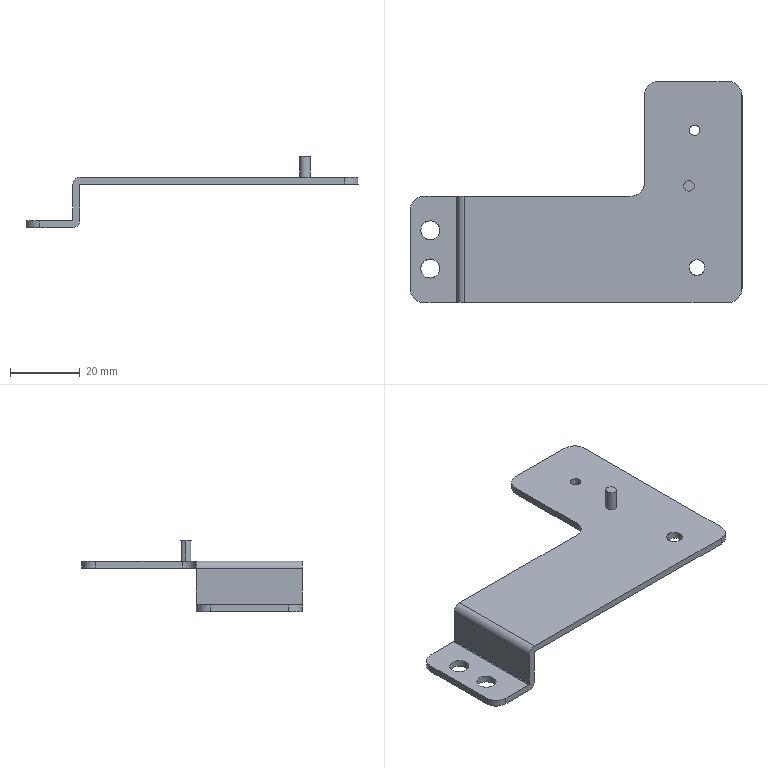Part | NX | features BREP 1 | 1 solid | 31 faces | box 95.45 x 63.5 x 20.5 mm | volume 8247 mm3 | cylinder 18 | plane 13 | commonest cylinder face diameters 8 x6 3 x4 0.3 x2 4.3 x2 4.5 x2 5.5 x2
STEP:
#1=CARTESIAN_POINT('',(-456.8,35.5,220.4));
#2=VERTEX_POINT('',#1);
#3=CARTESIAN_POINT('',(-456.8,35.5,226.4));
#4=VERTEX_POINT('',#3);
#5=CARTESIAN_POINT('',(-456.8,35.5,223.4));
#6=DIRECTION('',(0.,0.,1.));
#7=VECTOR('',#6,1000.);
#8=LINE('',#5,#7);
#9=EDGE_CURVE('',#2,#4,#8,.T.);
#10=ORIENTED_EDGE('',*,*,#9,.F.);
#11=CARTESIAN_POINT('',(-459.8,35.5,220.4));
#12=VERTEX_POINT('',#11);
#13=CARTESIAN_POINT('',(-458.3,35.5,220.4));
#14=DIRECTION('',(0.,0.,1.));
#15=DIRECTION('',(1.,0.,0.));
#16=AXIS2_PLACEMENT_3D('',#13,#14,#15);
#17=CIRCLE('',#16,1.5);
#18=EDGE_CURVE('',#2,#12,#17,.T.);
#19=ORIENTED_EDGE('',*,*,#18,.T.);
#20=CARTESIAN_POINT('',(-459.8,35.5,226.4));
#21=VERTEX_POINT('',#20);
#22=CARTESIAN_POINT('',(-459.8,35.5,223.4));
#23=DIRECTION('',(0.,0.,1.));
#24=VECTOR('',#23,1000.);
#25=LINE('',#22,#24);
#26=EDGE_CURVE('',#12,#21,#25,.T.);
#27=ORIENTED_EDGE('',*,*,#26,.T.);
#28=CARTESIAN_POINT('',(-458.3,35.5,226.4));
#29=DIRECTION('',(0.,0.,1.));
#30=DIRECTION('',(1.,0.,0.));
#31=AXIS2_PLACEMENT_3D('',#28,#29,#30);
#32=CIRCLE('',#31,1.5);
#33=EDGE_CURVE('',#4,#21,#32,.T.);
#34=ORIENTED_EDGE('',*,*,#33,.F.);
#35=EDGE_LOOP('',(#10,#19,#27,#34));
#36=FACE_BOUND('',#35,.T.);
#37=CARTESIAN_POINT('',(-458.3,35.5,223.4));
#38=DIRECTION('',(0.,0.,1.));
#39=DIRECTION('',(1.,0.,0.));
#40=AXIS2_PLACEMENT_3D('',#37,#38,#39);
#41=CYLINDRICAL_SURFACE('',#40,1.5);
#42=ADVANCED_FACE('',(#36),#41,.T.);
#43=ORIENTED_EDGE('',*,*,#26,.F.);
#44=CARTESIAN_POINT('',(-458.3,35.5,220.4));
#45=DIRECTION('',(0.,0.,1.));
#46=DIRECTION('',(1.,0.,0.));
#47=AXIS2_PLACEMENT_3D('',#44,#45,#46);
#48=CIRCLE('',#47,1.5);
#49=EDGE_CURVE('',#12,#2,#48,.T.);
#50=ORIENTED_EDGE('',*,*,#49,.T.);
#51=ORIENTED_EDGE('',*,*,#9,.T.);
#52=CARTESIAN_POINT('',(-458.3,35.5,226.4));
#53=DIRECTION('',(0.,0.,1.));
#54=DIRECTION('',(1.,0.,0.));
#55=AXIS2_PLACEMENT_3D('',#52,#53,#54);
#56=CIRCLE('',#55,1.5);
#57=EDGE_CURVE('',#21,#4,#56,.T.);
#58=ORIENTED_EDGE('',*,*,#57,.F.);
#59=EDGE_LOOP('',(#43,#50,#51,#58));
#60=FACE_BOUND('',#59,.T.);
#61=CARTESIAN_POINT('',(-458.3,35.5,223.4));
#62=DIRECTION('',(0.,0.,1.));
#63=DIRECTION('',(1.,0.,0.));
#64=AXIS2_PLACEMENT_3D('',#61,#62,#63);
#65=CYLINDRICAL_SURFACE('',#64,1.5);
#66=ADVANCED_FACE('',(#60),#65,.T.);
#67=ORIENTED_EDGE('',*,*,#33,.T.);
#68=ORIENTED_EDGE('',*,*,#57,.T.);
#69=EDGE_LOOP('',(#67,#68));
#70=FACE_BOUND('',#69,.T.);
#71=CARTESIAN_POINT('',(0.,0.,226.4));
#72=DIRECTION('',(0.,0.,1.));
#73=DIRECTION('',(1.,0.,0.));
#74=AXIS2_PLACEMENT_3D('',#71,#72,#73);
#75=PLANE('',#74);
#76=ADVANCED_FACE('',(#70),#75,.T.);
#77=CARTESIAN_POINT('',(-443.05,61.5,220.4));
#78=VERTEX_POINT('',#77);
#79=CARTESIAN_POINT('',(-447.05,65.5,220.4));
#80=VERTEX_POINT('',#79);
#81=CARTESIAN_POINT('',(-447.05,61.5,220.4));
#82=DIRECTION('',(0.,0.,1.));
#83=DIRECTION('',(1.,0.,0.));
#84=AXIS2_PLACEMENT_3D('',#81,#82,#83);
#85=CIRCLE('',#84,4.);
#86=EDGE_CURVE('',#78,#80,#85,.T.);
#87=ORIENTED_EDGE('',*,*,#86,.T.);
#88=CARTESIAN_POINT('',(-467.05,65.5,220.4));
#89=VERTEX_POINT('',#88);
#90=CARTESIAN_POINT('',(-457.05,65.5,220.4));
#91=DIRECTION('',(1.,0.,0.));
#92=VECTOR('',#91,1000.);
#93=LINE('',#90,#92);
#94=EDGE_CURVE('',#89,#80,#93,.T.);
#95=ORIENTED_EDGE('',*,*,#94,.F.);
#96=CARTESIAN_POINT('',(-471.05,61.5,220.4));
#97=VERTEX_POINT('',#96);
#98=CARTESIAN_POINT('',(-467.05,61.5,220.4));
#99=DIRECTION('',(0.,0.,1.));
#100=DIRECTION('',(1.,0.,0.));
#101=AXIS2_PLACEMENT_3D('',#98,#99,#100);
#102=CIRCLE('',#101,4.);
#103=EDGE_CURVE('',#89,#97,#102,.T.);
#104=ORIENTED_EDGE('',*,*,#103,.T.);
#105=CARTESIAN_POINT('',(-471.05,36.5,220.4));
#106=VERTEX_POINT('',#105);
#107=CARTESIAN_POINT('',(-471.05,49.,220.4));
#108=DIRECTION('',(0.,-1.,0.));
#109=VECTOR('',#108,1000.);
#110=LINE('',#107,#109);
#111=EDGE_CURVE('',#97,#106,#110,.T.);
#112=ORIENTED_EDGE('',*,*,#111,.T.);
#113=CARTESIAN_POINT('',(-475.05,32.5,220.4));
#114=VERTEX_POINT('',#113);
#115=CARTESIAN_POINT('',(-471.05,36.5,220.4));
#116=CARTESIAN_POINT('',(-471.05,36.108,220.4));
#117=CARTESIAN_POINT('',(-471.098,35.716,220.4));
#118=CARTESIAN_POINT('',(-471.194,35.332,220.4));
#119=CARTESIAN_POINT('',(-471.478,34.595,220.4));
#120=CARTESIAN_POINT('',(-471.932,33.949,220.4));
#121=CARTESIAN_POINT('',(-472.197,33.655,220.4));
#122=CARTESIAN_POINT('',(-472.794,33.139,220.4));
#123=CARTESIAN_POINT('',(-473.499,32.782,220.4));
#124=CARTESIAN_POINT('',(-473.871,32.647,220.4));
#125=CARTESIAN_POINT('',(-474.336,32.542,220.4));
#126=CARTESIAN_POINT('',(-474.807,32.506,220.4));
#127=CARTESIAN_POINT('',(-474.888,32.502,220.4));
#128=CARTESIAN_POINT('',(-474.969,32.5,220.4));
#129=CARTESIAN_POINT('',(-475.05,32.5,220.4));
#130=B_SPLINE_CURVE_WITH_KNOTS('',5,(#115,#116,#117,#118,#119,#120,#121,#122,#123,#124,#125,#126,#127,#128,#129),.UNSPECIFIED.,.F.,.F.,(6,3,3,3,6),(0.,0.3119,0.6238,0.9356,1.),.UNSPECIFIED.);
#131=EDGE_CURVE('',#106,#114,#130,.T.);
#132=ORIENTED_EDGE('',*,*,#131,.T.);
#133=CARTESIAN_POINT('',(-522.85,32.5,220.4));
#134=VERTEX_POINT('',#133);
#135=CARTESIAN_POINT('',(-494.95,32.5,220.4));
#136=DIRECTION('',(1.,0.,0.));
#137=VECTOR('',#136,1000.);
#138=LINE('',#135,#137);
#139=EDGE_CURVE('',#134,#114,#138,.T.);
#140=ORIENTED_EDGE('',*,*,#139,.F.);
#141=CARTESIAN_POINT('',(-522.85,2.,220.4));
#142=VERTEX_POINT('',#141);
#143=CARTESIAN_POINT('',(-522.85,17.25,220.4));
#144=DIRECTION('',(0.,1.,0.));
#145=VECTOR('',#144,1000.);
#146=LINE('',#143,#145);
#147=EDGE_CURVE('',#142,#134,#146,.T.);
#148=ORIENTED_EDGE('',*,*,#147,.F.);
#149=CARTESIAN_POINT('',(-447.05,2.,220.4));
#150=VERTEX_POINT('',#149);
#151=CARTESIAN_POINT('',(-480.95,2.,220.4));
#152=DIRECTION('',(-1.,0.,0.));
#153=VECTOR('',#152,1000.);
#154=LINE('',#151,#153);
#155=EDGE_CURVE('',#150,#142,#154,.T.);
#156=ORIENTED_EDGE('',*,*,#155,.F.);
#157=CARTESIAN_POINT('',(-443.05,6.,220.4));
#158=VERTEX_POINT('',#157);
#159=CARTESIAN_POINT('',(-447.05,6.,220.4));
#160=DIRECTION('',(0.,0.,1.));
#161=DIRECTION('',(1.,0.,0.));
#162=AXIS2_PLACEMENT_3D('',#159,#160,#161);
#163=CIRCLE('',#162,4.);
#164=EDGE_CURVE('',#150,#158,#163,.T.);
#165=ORIENTED_EDGE('',*,*,#164,.T.);
#166=CARTESIAN_POINT('',(-443.05,33.75,220.4));
#167=DIRECTION('',(0.,1.,0.));
#168=VECTOR('',#167,1000.);
#169=LINE('',#166,#168);
#170=EDGE_CURVE('',#158,#78,#169,.T.);
#171=ORIENTED_EDGE('',*,*,#170,.T.);
#172=EDGE_LOOP('',(#87,#95,#104,#112,#132,#140,#148,#156,#165,#171));
#173=FACE_BOUND('',#172,.T.);
#174=ORIENTED_EDGE('',*,*,#18,.F.);
#175=ORIENTED_EDGE('',*,*,#49,.F.);
#176=EDGE_LOOP('',(#174,#175));
#177=FACE_BOUND('',#176,.T.);
#178=CARTESIAN_POINT('',(-458.25,12.,220.4));
#179=VERTEX_POINT('',#178);
#180=CARTESIAN_POINT('',(-453.75,12.,220.4));
#181=VERTEX_POINT('',#180);
#182=CARTESIAN_POINT('',(-458.25,12.,220.4));
#183=CARTESIAN_POINT('',(-458.25,12.22,220.4));
#184=CARTESIAN_POINT('',(-458.223,12.441,220.4));
#185=CARTESIAN_POINT('',(-458.169,12.657,220.4));
#186=CARTESIAN_POINT('',(-458.009,13.071,220.4));
#187=CARTESIAN_POINT('',(-457.754,13.435,220.4));
#188=CARTESIAN_POINT('',(-457.605,13.6,220.4));
#189=CARTESIAN_POINT('',(-457.269,13.891,220.4));
#190=CARTESIAN_POINT('',(-456.873,14.092,220.4));
#191=CARTESIAN_POINT('',(-456.663,14.167,220.4));
#192=CARTESIAN_POINT('',(-456.23,14.265,220.4));
#193=CARTESIAN_POINT('',(-455.786,14.256,220.4));
#194=CARTESIAN_POINT('',(-455.565,14.224,220.4));
#195=CARTESIAN_POINT('',(-455.137,14.107,220.4));
#196=CARTESIAN_POINT('',(-454.749,13.89,220.4));
#197=CARTESIAN_POINT('',(-454.57,13.758,220.4));
#198=CARTESIAN_POINT('',(-454.247,13.453,220.4));
#199=CARTESIAN_POINT('',(-454.007,13.079,220.4));
#200=CARTESIAN_POINT('',(-453.911,12.878,220.4));
#201=CARTESIAN_POINT('',(-453.811,12.581,220.4));
#202=CARTESIAN_POINT('',(-453.764,12.273,220.4));
#203=CARTESIAN_POINT('',(-453.755,12.182,220.4));
#204=CARTESIAN_POINT('',(-453.75,12.091,220.4));
#205=CARTESIAN_POINT('',(-453.75,12.,220.4));
#206=B_SPLINE_CURVE_WITH_KNOTS('',5,(#182,#183,#184,#185,#186,#187,#188,#189,#190,#191,#192,#193,#194,#195,#196,#197,#198,#199,#200,#201,#202,#203,#204,#205),.UNSPECIFIED.,.F.,.F.,(6,3,3,3,3,3,3,6),(0.,0.156,0.3119,0.4679,0.6238,0.7798,0.9357,1.),.UNSPECIFIED.);
#207=EDGE_CURVE('',#179,#181,#206,.T.);
#208=ORIENTED_EDGE('',*,*,#207,.T.);
#209=CARTESIAN_POINT('',(-453.75,12.,220.4));
#210=CARTESIAN_POINT('',(-453.75,11.78,220.4));
#211=CARTESIAN_POINT('',(-453.777,11.559,220.4));
#212=CARTESIAN_POINT('',(-453.831,11.343,220.4));
#213=CARTESIAN_POINT('',(-453.991,10.929,220.4));
#214=CARTESIAN_POINT('',(-454.246,10.565,220.4));
#215=CARTESIAN_POINT('',(-454.395,10.4,220.4));
#216=CARTESIAN_POINT('',(-454.731,10.109,220.4));
#217=CARTESIAN_POINT('',(-455.127,9.908,220.4));
#218=CARTESIAN_POINT('',(-455.337,9.833,220.4));
#219=CARTESIAN_POINT('',(-455.77,9.735,220.4));
#220=CARTESIAN_POINT('',(-456.214,9.744,220.4));
#221=CARTESIAN_POINT('',(-456.435,9.776,220.4));
#222=CARTESIAN_POINT('',(-456.863,9.893,220.4));
#223=CARTESIAN_POINT('',(-457.251,10.11,220.4));
#224=CARTESIAN_POINT('',(-457.43,10.242,220.4));
#225=CARTESIAN_POINT('',(-457.753,10.547,220.4));
#226=CARTESIAN_POINT('',(-457.993,10.921,220.4));
#227=CARTESIAN_POINT('',(-458.089,11.122,220.4));
#228=CARTESIAN_POINT('',(-458.189,11.419,220.4));
#229=CARTESIAN_POINT('',(-458.236,11.727,220.4));
#230=CARTESIAN_POINT('',(-458.245,11.818,220.4));
#231=CARTESIAN_POINT('',(-458.25,11.909,220.4));
#232=CARTESIAN_POINT('',(-458.25,12.,220.4));
#233=B_SPLINE_CURVE_WITH_KNOTS('',5,(#209,#210,#211,#212,#213,#214,#215,#216,#217,#218,#219,#220,#221,#222,#223,#224,#225,#226,#227,#228,#229,#230,#231,#232),.UNSPECIFIED.,.F.,.F.,(6,3,3,3,3,3,3,6),(0.,0.156,0.3119,0.4679,0.6238,0.7798,0.9357,1.),.UNSPECIFIED.);
#234=EDGE_CURVE('',#181,#179,#233,.T.);
#235=ORIENTED_EDGE('',*,*,#234,.T.);
#236=EDGE_LOOP('',(#208,#235));
#237=FACE_BOUND('',#236,.T.);
#238=CARTESIAN_POINT('',(-457.991,52.219,220.4));
#239=VERTEX_POINT('',#238);
#240=CARTESIAN_POINT('',(-455.359,50.781,220.4));
#241=VERTEX_POINT('',#240);
#242=CARTESIAN_POINT('',(-457.991,52.219,220.4));
#243=CARTESIAN_POINT('',(-457.905,52.377,220.4));
#244=CARTESIAN_POINT('',(-457.795,52.522,220.4));
#245=CARTESIAN_POINT('',(-457.664,52.649,220.4));
#246=CARTESIAN_POINT('',(-457.368,52.861,220.4));
#247=CARTESIAN_POINT('',(-457.022,52.976,220.4));
#248=CARTESIAN_POINT('',(-456.842,53.007,220.4));
#249=CARTESIAN_POINT('',(-456.478,53.014,220.4));
#250=CARTESIAN_POINT('',(-456.128,52.914,220.4));
#251=CARTESIAN_POINT('',(-455.962,52.838,220.4));
#252=CARTESIAN_POINT('',(-455.658,52.639,220.4));
#253=CARTESIAN_POINT('',(-455.425,52.359,220.4));
#254=CARTESIAN_POINT('',(-455.331,52.202,220.4));
#255=CARTESIAN_POINT('',(-455.192,51.865,220.4));
#256=CARTESIAN_POINT('',(-455.159,51.503,220.4));
#257=CARTESIAN_POINT('',(-455.169,51.32,220.4));
#258=CARTESIAN_POINT('',(-455.216,51.1,220.4));
#259=CARTESIAN_POINT('',(-455.302,50.895,220.4));
#260=CARTESIAN_POINT('',(-455.319,50.856,220.4));
#261=CARTESIAN_POINT('',(-455.338,50.818,220.4));
#262=CARTESIAN_POINT('',(-455.359,50.781,220.4));
#263=B_SPLINE_CURVE_WITH_KNOTS('',5,(#242,#243,#244,#245,#246,#247,#248,#249,#250,#251,#252,#253,#254,#255,#256,#257,#258,#259,#260,#261,#262),.UNSPECIFIED.,.F.,.F.,(6,3,3,3,3,3,6),(0.,0.191,0.382,0.573,0.764,0.9549,1.),.UNSPECIFIED.);
#264=EDGE_CURVE('',#239,#241,#263,.T.);
#265=ORIENTED_EDGE('',*,*,#264,.T.);
#266=CARTESIAN_POINT('',(-455.359,50.781,220.4));
#267=CARTESIAN_POINT('',(-455.445,50.623,220.4));
#268=CARTESIAN_POINT('',(-455.555,50.478,220.4));
#269=CARTESIAN_POINT('',(-455.686,50.351,220.4));
#270=CARTESIAN_POINT('',(-455.982,50.139,220.4));
#271=CARTESIAN_POINT('',(-456.328,50.024,220.4));
#272=CARTESIAN_POINT('',(-456.508,49.993,220.4));
#273=CARTESIAN_POINT('',(-456.872,49.986,220.4));
#274=CARTESIAN_POINT('',(-457.222,50.086,220.4));
#275=CARTESIAN_POINT('',(-457.388,50.162,220.4));
#276=CARTESIAN_POINT('',(-457.692,50.361,220.4));
#277=CARTESIAN_POINT('',(-457.925,50.641,220.4));
#278=CARTESIAN_POINT('',(-458.019,50.798,220.4));
#279=CARTESIAN_POINT('',(-458.158,51.135,220.4));
#280=CARTESIAN_POINT('',(-458.191,51.497,220.4));
#281=CARTESIAN_POINT('',(-458.181,51.68,220.4));
#282=CARTESIAN_POINT('',(-458.134,51.9,220.4));
#283=CARTESIAN_POINT('',(-458.048,52.105,220.4));
#284=CARTESIAN_POINT('',(-458.031,52.144,220.4));
#285=CARTESIAN_POINT('',(-458.012,52.182,220.4));
#286=CARTESIAN_POINT('',(-457.991,52.219,220.4));
#287=B_SPLINE_CURVE_WITH_KNOTS('',5,(#266,#267,#268,#269,#270,#271,#272,#273,#274,#275,#276,#277,#278,#279,#280,#281,#282,#283,#284,#285,#286),.UNSPECIFIED.,.F.,.F.,(6,3,3,3,3,3,6),(0.,0.191,0.382,0.573,0.764,0.9549,1.),.UNSPECIFIED.);
#288=EDGE_CURVE('',#241,#239,#287,.T.);
#289=ORIENTED_EDGE('',*,*,#288,.T.);
#290=EDGE_LOOP('',(#265,#289));
#291=FACE_BOUND('',#290,.T.);
#292=CARTESIAN_POINT('',(0.,0.,220.4));
#293=DIRECTION('',(0.,0.,1.));
#294=DIRECTION('',(-1.,0.,0.));
#295=AXIS2_PLACEMENT_3D('',#292,#293,#294);
#296=PLANE('',#295);
#297=ADVANCED_FACE('',(#173,#177,#237,#291),#296,.T.);
#298=CARTESIAN_POINT('',(-535.433,11.75,205.9));
#299=VERTEX_POINT('',#298);
#300=CARTESIAN_POINT('',(-532.683,11.75,205.9));
#301=DIRECTION('',(0.,0.,-1.));
#302=DIRECTION('',(-1.,0.,0.));
#303=AXIS2_PLACEMENT_3D('',#300,#301,#302);
#304=CIRCLE('',#303,2.75);
#305=EDGE_CURVE('',#299,#299,#304,.T.);
#306=ORIENTED_EDGE('',*,*,#305,.F.);
#307=EDGE_LOOP('',(#306));
#308=FACE_BOUND('',#307,.T.);
#309=CARTESIAN_POINT('',(-535.433,22.75,205.9));
#310=VERTEX_POINT('',#309);
#311=CARTESIAN_POINT('',(-532.683,22.75,205.9));
#312=DIRECTION('',(0.,0.,-1.));
#313=DIRECTION('',(-1.,0.,0.));
#314=AXIS2_PLACEMENT_3D('',#311,#312,#313);
#315=CIRCLE('',#314,2.75);
#316=EDGE_CURVE('',#310,#310,#315,.T.);
#317=ORIENTED_EDGE('',*,*,#316,.F.);
#318=EDGE_LOOP('',(#317));
#319=FACE_BOUND('',#318,.T.);
#320=CARTESIAN_POINT('',(-538.5,28.5,205.9));
#321=VERTEX_POINT('',#320);
#322=CARTESIAN_POINT('',(-534.5,32.5,205.9));
#323=VERTEX_POINT('',#322);
#324=CARTESIAN_POINT('',(-534.5,28.5,205.9));
#325=DIRECTION('',(0.,0.,-1.));
#326=DIRECTION('',(-1.,0.,0.));
#327=AXIS2_PLACEMENT_3D('',#324,#325,#326);
#328=CIRCLE('',#327,4.);
#329=EDGE_CURVE('',#321,#323,#328,.T.);
#330=ORIENTED_EDGE('',*,*,#329,.T.);
#331=CARTESIAN_POINT('',(-525.15,32.5,205.9));
#332=VERTEX_POINT('',#331);
#333=CARTESIAN_POINT('',(-531.075,32.5,205.9));
#334=DIRECTION('',(-1.,0.,0.));
#335=VECTOR('',#334,1000.);
#336=LINE('',#333,#335);
#337=EDGE_CURVE('',#332,#323,#336,.T.);
#338=ORIENTED_EDGE('',*,*,#337,.F.);
#339=CARTESIAN_POINT('',(-525.15,2.,205.9));
#340=VERTEX_POINT('',#339);
#341=CARTESIAN_POINT('',(-525.15,0.,205.9));
#342=DIRECTION('',(0.,1.,0.));
#343=VECTOR('',#342,1000.);
#344=LINE('',#341,#343);
#345=EDGE_CURVE('',#340,#332,#344,.T.);
#346=ORIENTED_EDGE('',*,*,#345,.F.);
#347=CARTESIAN_POINT('',(-534.5,2.,205.9));
#348=VERTEX_POINT('',#347);
#349=CARTESIAN_POINT('',(-531.075,2.,205.9));
#350=DIRECTION('',(1.,0.,0.));
#351=VECTOR('',#350,1000.);
#352=LINE('',#349,#351);
#353=EDGE_CURVE('',#348,#340,#352,.T.);
#354=ORIENTED_EDGE('',*,*,#353,.F.);
#355=CARTESIAN_POINT('',(-538.5,6.,205.9));
#356=VERTEX_POINT('',#355);
#357=CARTESIAN_POINT('',(-534.5,6.,205.9));
#358=DIRECTION('',(0.,0.,-1.));
#359=DIRECTION('',(-1.,0.,0.));
#360=AXIS2_PLACEMENT_3D('',#357,#358,#359);
#361=CIRCLE('',#360,4.);
#362=EDGE_CURVE('',#348,#356,#361,.T.);
#363=ORIENTED_EDGE('',*,*,#362,.T.);
#364=CARTESIAN_POINT('',(-538.5,17.25,205.9));
#365=DIRECTION('',(0.,-1.,0.));
#366=VECTOR('',#365,1000.);
#367=LINE('',#364,#366);
#368=EDGE_CURVE('',#321,#356,#367,.T.);
#369=ORIENTED_EDGE('',*,*,#368,.F.);
#370=EDGE_LOOP('',(#330,#338,#346,#354,#363,#369));
#371=FACE_BOUND('',#370,.T.);
#372=CARTESIAN_POINT('',(-8.,0.,205.9));
#373=DIRECTION('',(0.,0.,-1.));
#374=DIRECTION('',(0.,1.,0.));
#375=AXIS2_PLACEMENT_3D('',#372,#373,#374);
#376=PLANE('',#375);
#377=ADVANCED_FACE('',(#308,#319,#371),#376,.T.);
#378=CARTESIAN_POINT('',(-538.5,28.5,207.9));
#379=VERTEX_POINT('',#378);
#380=CARTESIAN_POINT('',(-538.5,28.5,205.9));
#381=DIRECTION('',(0.,0.,1.));
#382=VECTOR('',#381,1000.);
#383=LINE('',#380,#382);
#384=EDGE_CURVE('',#321,#379,#383,.T.);
#385=ORIENTED_EDGE('',*,*,#384,.F.);
#386=ORIENTED_EDGE('',*,*,#368,.T.);
#387=CARTESIAN_POINT('',(-538.5,6.,207.9));
#388=VERTEX_POINT('',#387);
#389=CARTESIAN_POINT('',(-538.5,6.,206.9));
#390=DIRECTION('',(0.,0.,-1.));
#391=VECTOR('',#390,1000.);
#392=LINE('',#389,#391);
#393=EDGE_CURVE('',#388,#356,#392,.T.);
#394=ORIENTED_EDGE('',*,*,#393,.F.);
#395=CARTESIAN_POINT('',(-538.5,17.25,207.9));
#396=DIRECTION('',(0.,-1.,0.));
#397=VECTOR('',#396,1000.);
#398=LINE('',#395,#397);
#399=EDGE_CURVE('',#379,#388,#398,.T.);
#400=ORIENTED_EDGE('',*,*,#399,.F.);
#401=EDGE_LOOP('',(#385,#386,#394,#400));
#402=FACE_BOUND('',#401,.T.);
#403=CARTESIAN_POINT('',(-538.5,2.,205.9));
#404=DIRECTION('',(1.,0.,0.));
#405=DIRECTION('',(0.,-1.,0.));
#406=AXIS2_PLACEMENT_3D('',#403,#404,#405);
#407=PLANE('',#406);
#408=ADVANCED_FACE('',(#402),#407,.F.);
#409=ORIENTED_EDGE('',*,*,#384,.T.);
#410=CARTESIAN_POINT('',(-534.5,32.5,207.9));
#411=VERTEX_POINT('',#410);
#412=CARTESIAN_POINT('',(-534.5,28.5,207.9));
#413=DIRECTION('',(0.,0.,1.));
#414=DIRECTION('',(-1.,0.,0.));
#415=AXIS2_PLACEMENT_3D('',#412,#413,#414);
#416=CIRCLE('',#415,4.);
#417=EDGE_CURVE('',#411,#379,#416,.T.);
#418=ORIENTED_EDGE('',*,*,#417,.F.);
#419=CARTESIAN_POINT('',(-534.5,32.5,228.4));
#420=DIRECTION('',(0.,0.,-1.));
#421=VECTOR('',#420,1000.);
#422=LINE('',#419,#421);
#423=EDGE_CURVE('',#411,#323,#422,.T.);
#424=ORIENTED_EDGE('',*,*,#423,.T.);
#425=ORIENTED_EDGE('',*,*,#329,.F.);
#426=EDGE_LOOP('',(#409,#418,#424,#425));
#427=FACE_BOUND('',#426,.T.);
#428=CARTESIAN_POINT('',(-534.5,28.5,205.9));
#429=DIRECTION('',(0.,0.,1.));
#430=DIRECTION('',(-1.,0.,0.));
#431=AXIS2_PLACEMENT_3D('',#428,#429,#430);
#432=CYLINDRICAL_SURFACE('',#431,4.);
#433=ADVANCED_FACE('',(#427),#432,.T.);
#434=CARTESIAN_POINT('',(-523.,32.5,208.05));
#435=VERTEX_POINT('',#434);
#436=CARTESIAN_POINT('',(-523.,2.,208.05));
#437=VERTEX_POINT('',#436);
#438=CARTESIAN_POINT('',(-523.,0.,208.05));
#439=DIRECTION('',(0.,-1.,0.));
#440=VECTOR('',#439,1000.);
#441=LINE('',#438,#440);
#442=EDGE_CURVE('',#435,#437,#441,.T.);
#443=ORIENTED_EDGE('',*,*,#442,.F.);
#444=CARTESIAN_POINT('',(-523.,32.5,218.25));
#445=VERTEX_POINT('',#444);
#446=CARTESIAN_POINT('',(-523.,32.5,208.15));
#447=DIRECTION('',(0.,0.,-1.));
#448=VECTOR('',#447,1000.);
#449=LINE('',#446,#448);
#450=EDGE_CURVE('',#445,#435,#449,.T.);
#451=ORIENTED_EDGE('',*,*,#450,.F.);
#452=CARTESIAN_POINT('',(-523.,2.,218.25));
#453=VERTEX_POINT('',#452);
#454=CARTESIAN_POINT('',(-523.,0.,218.25));
#455=DIRECTION('',(0.,1.,0.));
#456=VECTOR('',#455,1000.);
#457=LINE('',#454,#456);
#458=EDGE_CURVE('',#453,#445,#457,.T.);
#459=ORIENTED_EDGE('',*,*,#458,.F.);
#460=CARTESIAN_POINT('',(-523.,2.,208.15));
#461=DIRECTION('',(0.,0.,1.));
#462=VECTOR('',#461,1000.);
#463=LINE('',#460,#462);
#464=EDGE_CURVE('',#437,#453,#463,.T.);
#465=ORIENTED_EDGE('',*,*,#464,.F.);
#466=EDGE_LOOP('',(#443,#451,#459,#465));
#467=FACE_BOUND('',#466,.T.);
#468=CARTESIAN_POINT('',(-523.,0.,0.));
#469=DIRECTION('',(1.,0.,0.));
#470=DIRECTION('',(0.,-1.,0.));
#471=AXIS2_PLACEMENT_3D('',#468,#469,#470);
#472=PLANE('',#471);
#473=ADVANCED_FACE('',(#467),#472,.T.);
#474=CARTESIAN_POINT('',(-525.15,2.,208.05));
#475=DIRECTION('',(0.,-1.,0.));
#476=DIRECTION('',(0.,0.,-1.));
#477=AXIS2_PLACEMENT_3D('',#474,#475,#476);
#478=CIRCLE('',#477,2.15);
#479=EDGE_CURVE('',#340,#437,#478,.T.);
#480=ORIENTED_EDGE('',*,*,#479,.F.);
#481=ORIENTED_EDGE('',*,*,#345,.T.);
#482=CARTESIAN_POINT('',(-525.15,32.5,208.05));
#483=DIRECTION('',(0.,1.,0.));
#484=DIRECTION('',(0.,0.,1.));
#485=AXIS2_PLACEMENT_3D('',#482,#483,#484);
#486=CIRCLE('',#485,2.15);
#487=EDGE_CURVE('',#435,#332,#486,.T.);
#488=ORIENTED_EDGE('',*,*,#487,.F.);
#489=ORIENTED_EDGE('',*,*,#442,.T.);
#490=EDGE_LOOP('',(#480,#481,#488,#489));
#491=FACE_BOUND('',#490,.T.);
#492=CARTESIAN_POINT('',(-525.15,0.,208.05));
#493=DIRECTION('',(0.,-1.,0.));
#494=DIRECTION('',(0.,0.,-1.));
#495=AXIS2_PLACEMENT_3D('',#492,#493,#494);
#496=CYLINDRICAL_SURFACE('',#495,2.15);
#497=ADVANCED_FACE('',(#491),#496,.T.);
#498=CARTESIAN_POINT('',(-534.5,2.,207.9));
#499=VERTEX_POINT('',#498);
#500=CARTESIAN_POINT('',(-534.5,2.,205.9));
#501=DIRECTION('',(0.,0.,1.));
#502=VECTOR('',#501,1000.);
#503=LINE('',#500,#502);
#504=EDGE_CURVE('',#348,#499,#503,.T.);
#505=ORIENTED_EDGE('',*,*,#504,.T.);
#506=CARTESIAN_POINT('',(-534.5,6.,207.9));
#507=DIRECTION('',(0.,0.,1.));
#508=DIRECTION('',(-1.,0.,0.));
#509=AXIS2_PLACEMENT_3D('',#506,#507,#508);
#510=CIRCLE('',#509,4.);
#511=EDGE_CURVE('',#388,#499,#510,.T.);
#512=ORIENTED_EDGE('',*,*,#511,.F.);
#513=ORIENTED_EDGE('',*,*,#393,.T.);
#514=ORIENTED_EDGE('',*,*,#362,.F.);
#515=EDGE_LOOP('',(#505,#512,#513,#514));
#516=FACE_BOUND('',#515,.T.);
#517=CARTESIAN_POINT('',(-534.5,6.,205.9));
#518=DIRECTION('',(0.,0.,-1.));
#519=DIRECTION('',(1.,0.,0.));
#520=AXIS2_PLACEMENT_3D('',#517,#518,#519);
#521=CYLINDRICAL_SURFACE('',#520,4.);
#522=ADVANCED_FACE('',(#516),#521,.T.);
#523=CARTESIAN_POINT('',(-532.683,9.,207.9));
#524=VERTEX_POINT('',#523);
#525=CARTESIAN_POINT('',(-532.683,11.75,207.9));
#526=DIRECTION('',(0.,0.,1.));
#527=DIRECTION('',(0.,-1.,0.));
#528=AXIS2_PLACEMENT_3D('',#525,#526,#527);
#529=CIRCLE('',#528,2.75);
#530=EDGE_CURVE('',#524,#524,#529,.T.);
#531=ORIENTED_EDGE('',*,*,#530,.F.);
#532=EDGE_LOOP('',(#531));
#533=FACE_BOUND('',#532,.T.);
#534=CARTESIAN_POINT('',(-532.683,20.,207.9));
#535=VERTEX_POINT('',#534);
#536=CARTESIAN_POINT('',(-532.683,22.75,207.9));
#537=DIRECTION('',(0.,0.,1.));
#538=DIRECTION('',(0.,-1.,0.));
#539=AXIS2_PLACEMENT_3D('',#536,#537,#538);
#540=CIRCLE('',#539,2.75);
#541=EDGE_CURVE('',#535,#535,#540,.T.);
#542=ORIENTED_EDGE('',*,*,#541,.F.);
#543=EDGE_LOOP('',(#542));
#544=FACE_BOUND('',#543,.T.);
#545=ORIENTED_EDGE('',*,*,#417,.T.);
#546=ORIENTED_EDGE('',*,*,#399,.T.);
#547=ORIENTED_EDGE('',*,*,#511,.T.);
#548=CARTESIAN_POINT('',(-525.15,2.,207.9));
#549=VERTEX_POINT('',#548);
#550=CARTESIAN_POINT('',(-531.075,2.,207.9));
#551=DIRECTION('',(1.,0.,0.));
#552=VECTOR('',#551,1000.);
#553=LINE('',#550,#552);
#554=EDGE_CURVE('',#499,#549,#553,.T.);
#555=ORIENTED_EDGE('',*,*,#554,.T.);
#556=CARTESIAN_POINT('',(-525.15,32.5,207.9));
#557=VERTEX_POINT('',#556);
#558=CARTESIAN_POINT('',(-525.15,17.25,207.9));
#559=DIRECTION('',(0.,-1.,0.));
#560=VECTOR('',#559,1000.);
#561=LINE('',#558,#560);
#562=EDGE_CURVE('',#557,#549,#561,.T.);
#563=ORIENTED_EDGE('',*,*,#562,.F.);
#564=CARTESIAN_POINT('',(-531.075,32.5,207.9));
#565=DIRECTION('',(-1.,0.,0.));
#566=VECTOR('',#565,1000.);
#567=LINE('',#564,#566);
#568=EDGE_CURVE('',#557,#411,#567,.T.);
#569=ORIENTED_EDGE('',*,*,#568,.T.);
#570=EDGE_LOOP('',(#545,#546,#547,#555,#563,#569));
#571=FACE_BOUND('',#570,.T.);
#572=CARTESIAN_POINT('',(-8.,0.,207.9));
#573=DIRECTION('',(0.,0.,-1.));
#574=DIRECTION('',(0.,1.,0.));
#575=AXIS2_PLACEMENT_3D('',#572,#573,#574);
#576=PLANE('',#575);
#577=ADVANCED_FACE('',(#533,#544,#571),#576,.F.);
#578=CARTESIAN_POINT('',(-525.,32.5,208.05));
#579=VERTEX_POINT('',#578);
#580=CARTESIAN_POINT('',(-525.15,32.5,208.05));
#581=DIRECTION('',(0.,-1.,0.));
#582=DIRECTION('',(1.,0.,0.));
#583=AXIS2_PLACEMENT_3D('',#580,#581,#582);
#584=CIRCLE('',#583,0.15);
#585=EDGE_CURVE('',#557,#579,#584,.T.);
#586=ORIENTED_EDGE('',*,*,#585,.F.);
#587=ORIENTED_EDGE('',*,*,#562,.T.);
#588=CARTESIAN_POINT('',(-525.,2.,208.05));
#589=VERTEX_POINT('',#588);
#590=CARTESIAN_POINT('',(-525.15,2.,208.05));
#591=DIRECTION('',(0.,1.,0.));
#592=DIRECTION('',(1.,0.,0.));
#593=AXIS2_PLACEMENT_3D('',#590,#591,#592);
#594=CIRCLE('',#593,0.15);
#595=EDGE_CURVE('',#589,#549,#594,.T.);
#596=ORIENTED_EDGE('',*,*,#595,.F.);
#597=CARTESIAN_POINT('',(-525.,2.,208.05));
#598=DIRECTION('',(0.,1.,0.));
#599=VECTOR('',#598,1000.);
#600=LINE('',#597,#599);
#601=EDGE_CURVE('',#589,#579,#600,.T.);
#602=ORIENTED_EDGE('',*,*,#601,.T.);
#603=EDGE_LOOP('',(#586,#587,#596,#602));
#604=FACE_BOUND('',#603,.T.);
#605=CARTESIAN_POINT('',(-525.15,2.,208.05));
#606=DIRECTION('',(0.,1.,0.));
#607=DIRECTION('',(1.,0.,0.));
#608=AXIS2_PLACEMENT_3D('',#605,#606,#607);
#609=CYLINDRICAL_SURFACE('',#608,0.15);
#610=ADVANCED_FACE('',(#604),#609,.F.);
#611=CARTESIAN_POINT('',(-525.,2.,218.25));
#612=VERTEX_POINT('',#611);
#613=CARTESIAN_POINT('',(-525.,2.,208.15));
#614=DIRECTION('',(0.,0.,1.));
#615=VECTOR('',#614,1000.);
#616=LINE('',#613,#615);
#617=EDGE_CURVE('',#589,#612,#616,.T.);
#618=ORIENTED_EDGE('',*,*,#617,.T.);
#619=CARTESIAN_POINT('',(-525.,32.5,218.25));
#620=VERTEX_POINT('',#619);
#621=CARTESIAN_POINT('',(-525.,17.25,218.25));
#622=DIRECTION('',(0.,-1.,0.));
#623=VECTOR('',#622,1000.);
#624=LINE('',#621,#623);
#625=EDGE_CURVE('',#620,#612,#624,.T.);
#626=ORIENTED_EDGE('',*,*,#625,.F.);
#627=CARTESIAN_POINT('',(-525.,32.5,208.15));
#628=DIRECTION('',(0.,0.,-1.));
#629=VECTOR('',#628,1000.);
#630=LINE('',#627,#629);
#631=EDGE_CURVE('',#620,#579,#630,.T.);
#632=ORIENTED_EDGE('',*,*,#631,.T.);
#633=ORIENTED_EDGE('',*,*,#601,.F.);
#634=EDGE_LOOP('',(#618,#626,#632,#633));
#635=FACE_BOUND('',#634,.T.);
#636=CARTESIAN_POINT('',(-525.,0.,0.));
#637=DIRECTION('',(1.,0.,0.));
#638=DIRECTION('',(0.,-1.,0.));
#639=AXIS2_PLACEMENT_3D('',#636,#637,#638);
#640=PLANE('',#639);
#641=ADVANCED_FACE('',(#635),#640,.F.);
#642=CARTESIAN_POINT('',(-522.85,32.5,218.25));
#643=DIRECTION('',(0.,1.,0.));
#644=DIRECTION('',(1.,0.,0.));
#645=AXIS2_PLACEMENT_3D('',#642,#643,#644);
#646=CIRCLE('',#645,2.15);
#647=EDGE_CURVE('',#620,#134,#646,.T.);
#648=ORIENTED_EDGE('',*,*,#647,.F.);
#649=ORIENTED_EDGE('',*,*,#625,.T.);
#650=CARTESIAN_POINT('',(-522.85,2.,218.25));
#651=DIRECTION('',(0.,-1.,0.));
#652=DIRECTION('',(1.,0.,0.));
#653=AXIS2_PLACEMENT_3D('',#650,#651,#652);
#654=CIRCLE('',#653,2.15);
#655=EDGE_CURVE('',#142,#612,#654,.T.);
#656=ORIENTED_EDGE('',*,*,#655,.F.);
#657=ORIENTED_EDGE('',*,*,#147,.T.);
#658=EDGE_LOOP('',(#648,#649,#656,#657));
#659=FACE_BOUND('',#658,.T.);
#660=CARTESIAN_POINT('',(-522.85,32.5,218.25));
#661=DIRECTION('',(0.,-1.,0.));
#662=DIRECTION('',(0.,0.,1.));
#663=AXIS2_PLACEMENT_3D('',#660,#661,#662);
#664=CYLINDRICAL_SURFACE('',#663,2.15);
#665=ADVANCED_FACE('',(#659),#664,.T.);
#666=CARTESIAN_POINT('',(-453.75,12.,218.4));
#667=VERTEX_POINT('',#666);
#668=CARTESIAN_POINT('',(-453.75,12.,211.4));
#669=DIRECTION('',(0.,0.,-1.));
#670=VECTOR('',#669,1000.);
#671=LINE('',#668,#670);
#672=EDGE_CURVE('',#181,#667,#671,.T.);
#673=ORIENTED_EDGE('',*,*,#672,.F.);
#674=ORIENTED_EDGE('',*,*,#207,.F.);
#675=CARTESIAN_POINT('',(-458.25,12.,218.4));
#676=VERTEX_POINT('',#675);
#677=CARTESIAN_POINT('',(-458.25,12.,211.4));
#678=DIRECTION('',(0.,0.,1.));
#679=VECTOR('',#678,1000.);
#680=LINE('',#677,#679);
#681=EDGE_CURVE('',#676,#179,#680,.T.);
#682=ORIENTED_EDGE('',*,*,#681,.F.);
#683=CARTESIAN_POINT('',(-456.,12.,218.4));
#684=DIRECTION('',(0.,0.,1.));
#685=DIRECTION('',(1.,0.,0.));
#686=AXIS2_PLACEMENT_3D('',#683,#684,#685);
#687=CIRCLE('',#686,2.25);
#688=EDGE_CURVE('',#667,#676,#687,.T.);
#689=ORIENTED_EDGE('',*,*,#688,.F.);
#690=EDGE_LOOP('',(#673,#674,#682,#689));
#691=FACE_BOUND('',#690,.T.);
#692=CARTESIAN_POINT('',(-456.,12.,211.4));
#693=DIRECTION('',(0.,0.,1.));
#694=DIRECTION('',(1.,0.,0.));
#695=AXIS2_PLACEMENT_3D('',#692,#693,#694);
#696=CYLINDRICAL_SURFACE('',#695,2.25);
#697=ADVANCED_FACE('',(#691),#696,.F.);
#698=ORIENTED_EDGE('',*,*,#681,.T.);
#699=ORIENTED_EDGE('',*,*,#234,.F.);
#700=ORIENTED_EDGE('',*,*,#672,.T.);
#701=CARTESIAN_POINT('',(-456.,12.,218.4));
#702=DIRECTION('',(0.,0.,1.));
#703=DIRECTION('',(1.,0.,0.));
#704=AXIS2_PLACEMENT_3D('',#701,#702,#703);
#705=CIRCLE('',#704,2.25);
#706=EDGE_CURVE('',#676,#667,#705,.T.);
#707=ORIENTED_EDGE('',*,*,#706,.F.);
#708=EDGE_LOOP('',(#698,#699,#700,#707));
#709=FACE_BOUND('',#708,.T.);
#710=CARTESIAN_POINT('',(-456.,12.,211.4));
#711=DIRECTION('',(0.,0.,1.));
#712=DIRECTION('',(-1.,0.,0.));
#713=AXIS2_PLACEMENT_3D('',#710,#711,#712);
#714=CYLINDRICAL_SURFACE('',#713,2.25);
#715=ADVANCED_FACE('',(#709),#714,.F.);
#716=CARTESIAN_POINT('',(-447.05,65.5,218.4));
#717=VERTEX_POINT('',#716);
#718=CARTESIAN_POINT('',(-447.05,65.5,219.4));
#719=DIRECTION('',(0.,0.,1.));
#720=VECTOR('',#719,1000.);
#721=LINE('',#718,#720);
#722=EDGE_CURVE('',#717,#80,#721,.T.);
#723=ORIENTED_EDGE('',*,*,#722,.F.);
#724=CARTESIAN_POINT('',(-467.05,65.5,218.4));
#725=VERTEX_POINT('',#724);
#726=CARTESIAN_POINT('',(-457.05,65.5,218.4));
#727=DIRECTION('',(1.,0.,0.));
#728=VECTOR('',#727,1000.);
#729=LINE('',#726,#728);
#730=EDGE_CURVE('',#725,#717,#729,.T.);
#731=ORIENTED_EDGE('',*,*,#730,.F.);
#732=CARTESIAN_POINT('',(-467.05,65.5,219.4));
#733=DIRECTION('',(0.,0.,-1.));
#734=VECTOR('',#733,1000.);
#735=LINE('',#732,#734);
#736=EDGE_CURVE('',#89,#725,#735,.T.);
#737=ORIENTED_EDGE('',*,*,#736,.F.);
#738=ORIENTED_EDGE('',*,*,#94,.T.);
#739=EDGE_LOOP('',(#723,#731,#737,#738));
#740=FACE_BOUND('',#739,.T.);
#741=CARTESIAN_POINT('',(-294.174,65.5,217.465));
#742=DIRECTION('',(0.,1.,0.));
#743=DIRECTION('',(-1.,0.,0.));
#744=AXIS2_PLACEMENT_3D('',#741,#742,#743);
#745=PLANE('',#744);
#746=ADVANCED_FACE('',(#740),#745,.T.);
#747=ORIENTED_EDGE('',*,*,#736,.T.);
#748=CARTESIAN_POINT('',(-471.05,61.5,218.4));
#749=VERTEX_POINT('',#748);
#750=CARTESIAN_POINT('',(-467.05,61.5,218.4));
#751=DIRECTION('',(0.,0.,-1.));
#752=DIRECTION('',(1.,0.,0.));
#753=AXIS2_PLACEMENT_3D('',#750,#751,#752);
#754=CIRCLE('',#753,4.);
#755=EDGE_CURVE('',#749,#725,#754,.T.);
#756=ORIENTED_EDGE('',*,*,#755,.F.);
#757=CARTESIAN_POINT('',(-471.05,61.5,220.4));
#758=DIRECTION('',(0.,0.,1.));
#759=VECTOR('',#758,1000.);
#760=LINE('',#757,#759);
#761=EDGE_CURVE('',#749,#97,#760,.T.);
#762=ORIENTED_EDGE('',*,*,#761,.T.);
#763=ORIENTED_EDGE('',*,*,#103,.F.);
#764=EDGE_LOOP('',(#747,#756,#762,#763));
#765=FACE_BOUND('',#764,.T.);
#766=CARTESIAN_POINT('',(-467.05,61.5,220.4));
#767=DIRECTION('',(0.,0.,1.));
#768=DIRECTION('',(1.,0.,0.));
#769=AXIS2_PLACEMENT_3D('',#766,#767,#768);
#770=CYLINDRICAL_SURFACE('',#769,4.);
#771=ADVANCED_FACE('',(#765),#770,.T.);
#772=ORIENTED_EDGE('',*,*,#761,.F.);
#773=CARTESIAN_POINT('',(-471.05,36.5,218.4));
#774=VERTEX_POINT('',#773);
#775=CARTESIAN_POINT('',(-471.05,49.,218.4));
#776=DIRECTION('',(0.,-1.,0.));
#777=VECTOR('',#776,1000.);
#778=LINE('',#775,#777);
#779=EDGE_CURVE('',#749,#774,#778,.T.);
#780=ORIENTED_EDGE('',*,*,#779,.T.);
#781=CARTESIAN_POINT('',(-471.05,36.5,219.4));
#782=DIRECTION('',(0.,-0.000000002,-1.));
#783=VECTOR('',#782,1000.);
#784=LINE('',#781,#783);
#785=EDGE_CURVE('',#106,#774,#784,.T.);
#786=ORIENTED_EDGE('',*,*,#785,.F.);
#787=ORIENTED_EDGE('',*,*,#111,.F.);
#788=EDGE_LOOP('',(#772,#780,#786,#787));
#789=FACE_BOUND('',#788,.T.);
#790=CARTESIAN_POINT('',(-471.05,93.,220.4));
#791=DIRECTION('',(1.,0.,0.));
#792=DIRECTION('',(0.,-1.,0.));
#793=AXIS2_PLACEMENT_3D('',#790,#791,#792);
#794=PLANE('',#793);
#795=ADVANCED_FACE('',(#789),#794,.F.);
#796=CARTESIAN_POINT('',(-475.05,32.5,218.4));
#797=VERTEX_POINT('',#796);
#798=CARTESIAN_POINT('',(-475.05,32.5,220.4));
#799=DIRECTION('',(0.,0.,1.));
#800=VECTOR('',#799,1000.);
#801=LINE('',#798,#800);
#802=EDGE_CURVE('',#797,#114,#801,.T.);
#803=ORIENTED_EDGE('',*,*,#802,.T.);
#804=ORIENTED_EDGE('',*,*,#131,.F.);
#805=ORIENTED_EDGE('',*,*,#785,.T.);
#806=CARTESIAN_POINT('',(-475.05,36.5,218.4));
#807=DIRECTION('',(0.,0.,1.));
#808=DIRECTION('',(1.,0.,0.));
#809=AXIS2_PLACEMENT_3D('',#806,#807,#808);
#810=CIRCLE('',#809,4.);
#811=EDGE_CURVE('',#797,#774,#810,.T.);
#812=ORIENTED_EDGE('',*,*,#811,.F.);
#813=EDGE_LOOP('',(#803,#804,#805,#812));
#814=FACE_BOUND('',#813,.T.);
#815=CARTESIAN_POINT('',(-475.05,36.5,220.4));
#816=DIRECTION('',(0.,0.,1.));
#817=DIRECTION('',(-1.,0.,0.));
#818=AXIS2_PLACEMENT_3D('',#815,#816,#817);
#819=CYLINDRICAL_SURFACE('',#818,4.);
#820=ADVANCED_FACE('',(#814),#819,.F.);
#821=ORIENTED_EDGE('',*,*,#802,.F.);
#822=CARTESIAN_POINT('',(-522.85,32.5,218.4));
#823=VERTEX_POINT('',#822);
#824=CARTESIAN_POINT('',(-494.95,32.5,218.4));
#825=DIRECTION('',(1.,0.,0.));
#826=VECTOR('',#825,1000.);
#827=LINE('',#824,#826);
#828=EDGE_CURVE('',#823,#797,#827,.T.);
#829=ORIENTED_EDGE('',*,*,#828,.F.);
#830=CARTESIAN_POINT('',(-522.85,32.5,218.25));
#831=DIRECTION('',(0.,-1.,0.));
#832=DIRECTION('',(0.,0.,1.));
#833=AXIS2_PLACEMENT_3D('',#830,#831,#832);
#834=CIRCLE('',#833,0.15);
#835=EDGE_CURVE('',#823,#445,#834,.T.);
#836=ORIENTED_EDGE('',*,*,#835,.T.);
#837=ORIENTED_EDGE('',*,*,#450,.T.);
#838=ORIENTED_EDGE('',*,*,#487,.T.);
#839=ORIENTED_EDGE('',*,*,#337,.T.);
#840=ORIENTED_EDGE('',*,*,#423,.F.);
#841=ORIENTED_EDGE('',*,*,#568,.F.);
#842=ORIENTED_EDGE('',*,*,#585,.T.);
#843=ORIENTED_EDGE('',*,*,#631,.F.);
#844=ORIENTED_EDGE('',*,*,#647,.T.);
#845=ORIENTED_EDGE('',*,*,#139,.T.);
#846=EDGE_LOOP('',(#821,#829,#836,#837,#838,#839,#840,#841,#842,#843,#844,#845));
#847=FACE_BOUND('',#846,.T.);
#848=CARTESIAN_POINT('',(-471.05,32.5,218.4));
#849=DIRECTION('',(0.,1.,0.));
#850=DIRECTION('',(-1.,0.,0.));
#851=AXIS2_PLACEMENT_3D('',#848,#849,#850);
#852=PLANE('',#851);
#853=ADVANCED_FACE('',(#847),#852,.T.);
#854=CARTESIAN_POINT('',(-522.85,2.,218.4));
#855=VERTEX_POINT('',#854);
#856=CARTESIAN_POINT('',(-522.85,2.,218.25));
#857=DIRECTION('',(0.,1.,0.));
#858=DIRECTION('',(0.,0.,-1.));
#859=AXIS2_PLACEMENT_3D('',#856,#857,#858);
#860=CIRCLE('',#859,0.15);
#861=EDGE_CURVE('',#453,#855,#860,.T.);
#862=ORIENTED_EDGE('',*,*,#861,.F.);
#863=ORIENTED_EDGE('',*,*,#458,.T.);
#864=ORIENTED_EDGE('',*,*,#835,.F.);
#865=CARTESIAN_POINT('',(-522.85,0.,218.4));
#866=DIRECTION('',(0.,-1.,0.));
#867=VECTOR('',#866,1000.);
#868=LINE('',#865,#867);
#869=EDGE_CURVE('',#823,#855,#868,.T.);
#870=ORIENTED_EDGE('',*,*,#869,.T.);
#871=EDGE_LOOP('',(#862,#863,#864,#870));
#872=FACE_BOUND('',#871,.T.);
#873=CARTESIAN_POINT('',(-522.85,0.,218.25));
#874=DIRECTION('',(0.,-1.,0.));
#875=DIRECTION('',(0.,0.,-1.));
#876=AXIS2_PLACEMENT_3D('',#873,#874,#875);
#877=CYLINDRICAL_SURFACE('',#876,0.15);
#878=ADVANCED_FACE('',(#872),#877,.F.);
#879=CARTESIAN_POINT('',(-447.05,2.,218.4));
#880=VERTEX_POINT('',#879);
#881=CARTESIAN_POINT('',(-447.05,2.,219.4));
#882=DIRECTION('',(0.,0.,-1.));
#883=VECTOR('',#882,1000.);
#884=LINE('',#881,#883);
#885=EDGE_CURVE('',#150,#880,#884,.T.);
#886=ORIENTED_EDGE('',*,*,#885,.F.);
#887=ORIENTED_EDGE('',*,*,#155,.T.);
#888=ORIENTED_EDGE('',*,*,#655,.T.);
#889=ORIENTED_EDGE('',*,*,#617,.F.);
#890=ORIENTED_EDGE('',*,*,#595,.T.);
#891=ORIENTED_EDGE('',*,*,#554,.F.);
#892=ORIENTED_EDGE('',*,*,#504,.F.);
#893=ORIENTED_EDGE('',*,*,#353,.T.);
#894=ORIENTED_EDGE('',*,*,#479,.T.);
#895=ORIENTED_EDGE('',*,*,#464,.T.);
#896=ORIENTED_EDGE('',*,*,#861,.T.);
#897=CARTESIAN_POINT('',(-480.95,2.,218.4));
#898=DIRECTION('',(-1.,0.,0.));
#899=VECTOR('',#898,1000.);
#900=LINE('',#897,#899);
#901=EDGE_CURVE('',#880,#855,#900,.T.);
#902=ORIENTED_EDGE('',*,*,#901,.F.);
#903=EDGE_LOOP('',(#886,#887,#888,#889,#890,#891,#892,#893,#894,#895,#896,#902));
#904=FACE_BOUND('',#903,.T.);
#905=CARTESIAN_POINT('',(-511.5,2.,218.4));
#906=DIRECTION('',(0.,-1.,0.));
#907=DIRECTION('',(0.,0.,1.));
#908=AXIS2_PLACEMENT_3D('',#905,#906,#907);
#909=PLANE('',#908);
#910=ADVANCED_FACE('',(#904),#909,.T.);
#911=CARTESIAN_POINT('',(-443.05,6.,218.4));
#912=VERTEX_POINT('',#911);
#913=CARTESIAN_POINT('',(-443.05,6.,218.4));
#914=DIRECTION('',(0.,0.,1.));
#915=VECTOR('',#914,1000.);
#916=LINE('',#913,#915);
#917=EDGE_CURVE('',#912,#158,#916,.T.);
#918=ORIENTED_EDGE('',*,*,#917,.T.);
#919=ORIENTED_EDGE('',*,*,#164,.F.);
#920=ORIENTED_EDGE('',*,*,#885,.T.);
#921=CARTESIAN_POINT('',(-447.05,6.,218.4));
#922=DIRECTION('',(0.,0.,-1.));
#923=DIRECTION('',(-1.,0.,0.));
#924=AXIS2_PLACEMENT_3D('',#921,#922,#923);
#925=CIRCLE('',#924,4.);
#926=EDGE_CURVE('',#912,#880,#925,.T.);
#927=ORIENTED_EDGE('',*,*,#926,.F.);
#928=EDGE_LOOP('',(#918,#919,#920,#927));
#929=FACE_BOUND('',#928,.T.);
#930=CARTESIAN_POINT('',(-447.05,6.,218.4));
#931=DIRECTION('',(0.,0.,-1.));
#932=DIRECTION('',(1.,0.,0.));
#933=AXIS2_PLACEMENT_3D('',#930,#931,#932);
#934=CYLINDRICAL_SURFACE('',#933,4.);
#935=ADVANCED_FACE('',(#929),#934,.T.);
#936=CARTESIAN_POINT('',(-443.05,61.5,218.4));
#937=VERTEX_POINT('',#936);
#938=CARTESIAN_POINT('',(-443.05,61.5,219.4));
#939=DIRECTION('',(0.,0.,-1.));
#940=VECTOR('',#939,1000.);
#941=LINE('',#938,#940);
#942=EDGE_CURVE('',#78,#937,#941,.T.);
#943=ORIENTED_EDGE('',*,*,#942,.F.);
#944=ORIENTED_EDGE('',*,*,#170,.F.);
#945=ORIENTED_EDGE('',*,*,#917,.F.);
#946=CARTESIAN_POINT('',(-443.05,33.75,218.4));
#947=DIRECTION('',(0.,1.,0.));
#948=VECTOR('',#947,1000.);
#949=LINE('',#946,#948);
#950=EDGE_CURVE('',#912,#937,#949,.T.);
#951=ORIENTED_EDGE('',*,*,#950,.T.);
#952=EDGE_LOOP('',(#943,#944,#945,#951));
#953=FACE_BOUND('',#952,.T.);
#954=CARTESIAN_POINT('',(-443.05,42.75,220.4));
#955=DIRECTION('',(-1.,0.,0.));
#956=DIRECTION('',(0.,0.,-1.));
#957=AXIS2_PLACEMENT_3D('',#954,#955,#956);
#958=PLANE('',#957);
#959=ADVANCED_FACE('',(#953),#958,.F.);
#960=ORIENTED_EDGE('',*,*,#942,.T.);
#961=CARTESIAN_POINT('',(-447.05,61.5,218.4));
#962=DIRECTION('',(0.,0.,-1.));
#963=DIRECTION('',(1.,0.,0.));
#964=AXIS2_PLACEMENT_3D('',#961,#962,#963);
#965=CIRCLE('',#964,4.);
#966=EDGE_CURVE('',#717,#937,#965,.T.);
#967=ORIENTED_EDGE('',*,*,#966,.F.);
#968=ORIENTED_EDGE('',*,*,#722,.T.);
#969=ORIENTED_EDGE('',*,*,#86,.F.);
#970=EDGE_LOOP('',(#960,#967,#968,#969));
#971=FACE_BOUND('',#970,.T.);
#972=CARTESIAN_POINT('',(-447.05,61.5,217.465));
#973=DIRECTION('',(0.,0.,1.));
#974=DIRECTION('',(1.,0.,0.));
#975=AXIS2_PLACEMENT_3D('',#972,#973,#974);
#976=CYLINDRICAL_SURFACE('',#975,4.);
#977=ADVANCED_FACE('',(#971),#976,.T.);
#978=ORIENTED_EDGE('',*,*,#966,.T.);
#979=ORIENTED_EDGE('',*,*,#950,.F.);
#980=ORIENTED_EDGE('',*,*,#926,.T.);
#981=ORIENTED_EDGE('',*,*,#901,.T.);
#982=ORIENTED_EDGE('',*,*,#869,.F.);
#983=ORIENTED_EDGE('',*,*,#828,.T.);
#984=ORIENTED_EDGE('',*,*,#811,.T.);
#985=ORIENTED_EDGE('',*,*,#779,.F.);
#986=ORIENTED_EDGE('',*,*,#755,.T.);
#987=ORIENTED_EDGE('',*,*,#730,.T.);
#988=EDGE_LOOP('',(#978,#979,#980,#981,#982,#983,#984,#985,#986,#987));
#989=FACE_BOUND('',#988,.T.);
#990=ORIENTED_EDGE('',*,*,#706,.T.);
#991=ORIENTED_EDGE('',*,*,#688,.T.);
#992=EDGE_LOOP('',(#990,#991));
#993=FACE_BOUND('',#992,.T.);
#994=CARTESIAN_POINT('',(-457.991,52.219,218.4));
#995=VERTEX_POINT('',#994);
#996=CARTESIAN_POINT('',(-455.359,50.781,218.4));
#997=VERTEX_POINT('',#996);
#998=CARTESIAN_POINT('',(-456.675,51.5,218.4));
#999=DIRECTION('',(0.,0.,1.));
#1000=DIRECTION('',(1.,0.,0.));
#1001=AXIS2_PLACEMENT_3D('',#998,#999,#1000);
#1002=CIRCLE('',#1001,1.5);
#1003=EDGE_CURVE('',#995,#997,#1002,.T.);
#1004=ORIENTED_EDGE('',*,*,#1003,.T.);
#1005=CARTESIAN_POINT('',(-456.675,51.5,218.4));
#1006=DIRECTION('',(0.,0.,1.));
#1007=DIRECTION('',(1.,0.,0.));
#1008=AXIS2_PLACEMENT_3D('',#1005,#1006,#1007);
#1009=CIRCLE('',#1008,1.5);
#1010=EDGE_CURVE('',#997,#995,#1009,.T.);
#1011=ORIENTED_EDGE('',*,*,#1010,.T.);
#1012=EDGE_LOOP('',(#1004,#1011));
#1013=FACE_BOUND('',#1012,.T.);
#1014=CARTESIAN_POINT('',(0.,0.,218.4));
#1015=DIRECTION('',(0.,0.,1.));
#1016=DIRECTION('',(-1.,0.,0.));
#1017=AXIS2_PLACEMENT_3D('',#1014,#1015,#1016);
#1018=PLANE('',#1017);
#1019=ADVANCED_FACE('',(#989,#993,#1013),#1018,.F.);
#1020=CARTESIAN_POINT('',(-457.991,52.219,219.4));
#1021=DIRECTION('',(0.,0.,-1.));
#1022=VECTOR('',#1021,1000.);
#1023=LINE('',#1020,#1022);
#1024=EDGE_CURVE('',#239,#995,#1023,.T.);
#1025=ORIENTED_EDGE('',*,*,#1024,.T.);
#1026=ORIENTED_EDGE('',*,*,#1010,.F.);
#1027=CARTESIAN_POINT('',(-455.359,50.781,219.4));
#1028=DIRECTION('',(0.,0.,-1.));
#1029=VECTOR('',#1028,1000.);
#1030=LINE('',#1027,#1029);
#1031=EDGE_CURVE('',#241,#997,#1030,.T.);
#1032=ORIENTED_EDGE('',*,*,#1031,.F.);
#1033=ORIENTED_EDGE('',*,*,#264,.F.);
#1034=EDGE_LOOP('',(#1025,#1026,#1032,#1033));
#1035=FACE_BOUND('',#1034,.T.);
#1036=CARTESIAN_POINT('',(-456.675,51.5,219.4));
#1037=DIRECTION('',(0.,0.,-1.));
#1038=DIRECTION('',(-0.8776,0.4794,0.));
#1039=AXIS2_PLACEMENT_3D('',#1036,#1037,#1038);
#1040=CYLINDRICAL_SURFACE('',#1039,1.5);
#1041=ADVANCED_FACE('',(#1035),#1040,.F.);
#1042=ORIENTED_EDGE('',*,*,#1031,.T.);
#1043=ORIENTED_EDGE('',*,*,#1003,.F.);
#1044=ORIENTED_EDGE('',*,*,#1024,.F.);
#1045=ORIENTED_EDGE('',*,*,#288,.F.);
#1046=EDGE_LOOP('',(#1042,#1043,#1044,#1045));
#1047=FACE_BOUND('',#1046,.T.);
#1048=CARTESIAN_POINT('',(-456.675,51.5,219.4));
#1049=DIRECTION('',(0.,0.,-1.));
#1050=DIRECTION('',(0.8776,-0.4794,0.));
#1051=AXIS2_PLACEMENT_3D('',#1048,#1049,#1050);
#1052=CYLINDRICAL_SURFACE('',#1051,1.5);
#1053=ADVANCED_FACE('',(#1047),#1052,.F.);
#1054=ORIENTED_EDGE('',*,*,#316,.T.);
#1055=EDGE_LOOP('',(#1054));
#1056=FACE_BOUND('',#1055,.T.);
#1057=ORIENTED_EDGE('',*,*,#541,.T.);
#1058=EDGE_LOOP('',(#1057));
#1059=FACE_BOUND('',#1058,.T.);
#1060=CARTESIAN_POINT('',(-532.683,22.75,202.4));
#1061=DIRECTION('',(0.,0.,1.));
#1062=DIRECTION('',(1.,0.,0.));
#1063=AXIS2_PLACEMENT_3D('',#1060,#1061,#1062);
#1064=CYLINDRICAL_SURFACE('',#1063,2.75);
#1065=ADVANCED_FACE('',(#1056,#1059),#1064,.F.);
#1066=ORIENTED_EDGE('',*,*,#305,.T.);
#1067=EDGE_LOOP('',(#1066));
#1068=FACE_BOUND('',#1067,.T.);
#1069=ORIENTED_EDGE('',*,*,#530,.T.);
#1070=EDGE_LOOP('',(#1069));
#1071=FACE_BOUND('',#1070,.T.);
#1072=CARTESIAN_POINT('',(-532.683,11.75,202.4));
#1073=DIRECTION('',(0.,0.,1.));
#1074=DIRECTION('',(1.,0.,0.));
#1075=AXIS2_PLACEMENT_3D('',#1072,#1073,#1074);
#1076=CYLINDRICAL_SURFACE('',#1075,2.75);
#1077=ADVANCED_FACE('',(#1068,#1071),#1076,.F.);
#1078=CLOSED_SHELL('',(#42,#66,#76,#297,#377,#408,#433,#473,#497,#522,#577,#610,#641,#665,#697,#715,#746,#771,#795,#820,#853,#878,#910,#935,#959,#977,#1019,#1041,#1053,#1065,#1077));
#1079=MANIFOLD_SOLID_BREP('',#1078);
#1080=(LENGTH_UNIT()NAMED_UNIT(*)SI_UNIT(.MILLI.,.METRE.));
#1081=UNCERTAINTY_MEASURE_WITH_UNIT(LENGTH_MEASURE(0.00001),#1080,'','');
#1082=(NAMED_UNIT(*)PLANE_ANGLE_UNIT()SI_UNIT($,.RADIAN.));
#1083=(NAMED_UNIT(*)SI_UNIT($,.STERADIAN.)SOLID_ANGLE_UNIT());
#1084=(GEOMETRIC_REPRESENTATION_CONTEXT(3)GLOBAL_UNCERTAINTY_ASSIGNED_CONTEXT((#1081))GLOBAL_UNIT_ASSIGNED_CONTEXT((#1080,#1082,#1083))REPRESENTATION_CONTEXT('',''));
#1085=ADVANCED_BREP_SHAPE_REPRESENTATION('',(#1079),#1084);